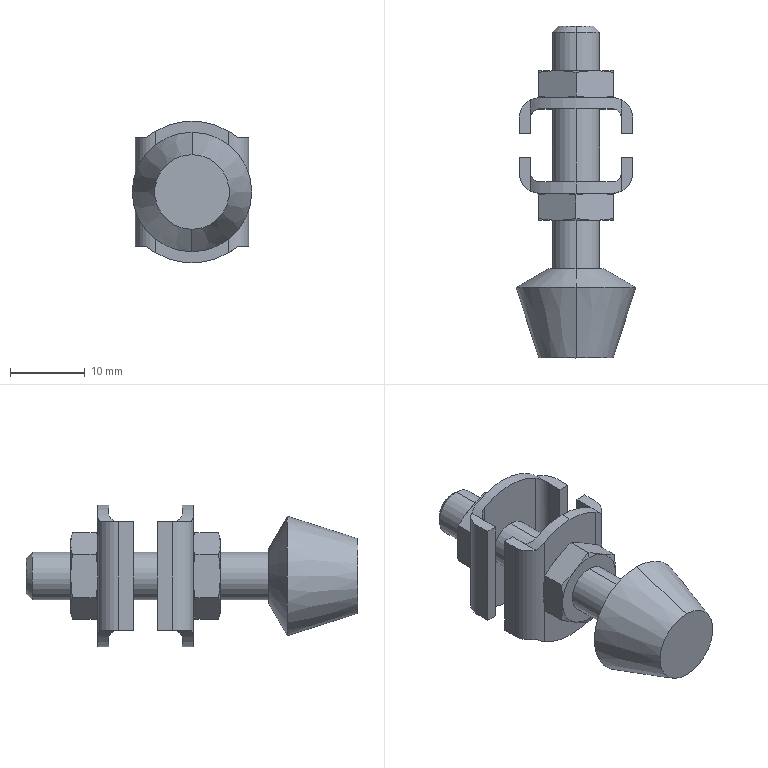Part | SolidWorks | features BaseBody 1 | 1 solid | 100 faces | box 16 x 44.45 x 19 mm | volume 3867 mm3 | plane 47 | cone 33 | cylinder 20 | commonest cylinder face diameters 6.35 x6 19 x6 2.5 x4 5.5 x4